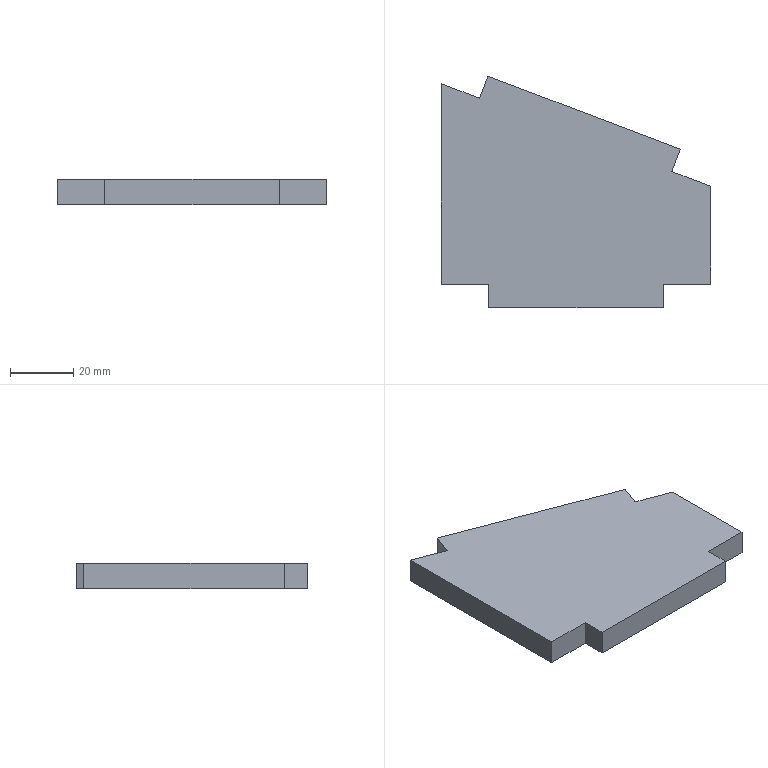Part | SolidWorks | features FlatPattern 1, SMBaseFlange 1, SheetMetal 1 | 1 solid | 14 faces | box 85 x 73.23 x 8 mm | volume 39231 mm3 | plane 14
STEP:
#1=CARTESIAN_POINT('',(162.814,62.221,0.));
#2=VERTEX_POINT('',#1);
#3=CARTESIAN_POINT('',(150.814,66.792,0.));
#4=VERTEX_POINT('',#3);
#5=CARTESIAN_POINT('',(162.814,62.221,0.));
#6=DIRECTION('',(-0.9345,0.3559,0.));
#7=VECTOR('',#6,1000.);
#8=LINE('',#5,#7);
#9=EDGE_CURVE('',#2,#4,#8,.T.);
#10=ORIENTED_EDGE('',*,*,#9,.T.);
#11=CARTESIAN_POINT('',(150.814,66.792,8.));
#12=VERTEX_POINT('',#11);
#13=CARTESIAN_POINT('',(150.814,66.792,8.));
#14=DIRECTION('',(0.,0.,-1.));
#15=VECTOR('',#14,1000.);
#16=LINE('',#13,#15);
#17=EDGE_CURVE('',#12,#4,#16,.T.);
#18=ORIENTED_EDGE('',*,*,#17,.F.);
#19=CARTESIAN_POINT('',(162.814,62.221,8.));
#20=VERTEX_POINT('',#19);
#21=CARTESIAN_POINT('',(162.814,62.221,8.));
#22=DIRECTION('',(-0.9345,0.3559,0.));
#23=VECTOR('',#22,1000.);
#24=LINE('',#21,#23);
#25=EDGE_CURVE('',#20,#12,#24,.T.);
#26=ORIENTED_EDGE('',*,*,#25,.F.);
#27=CARTESIAN_POINT('',(162.814,62.221,8.));
#28=DIRECTION('',(0.,0.,-1.));
#29=VECTOR('',#28,1000.);
#30=LINE('',#27,#29);
#31=EDGE_CURVE('',#20,#2,#30,.T.);
#32=ORIENTED_EDGE('',*,*,#31,.T.);
#33=EDGE_LOOP('',(#10,#18,#26,#32));
#34=FACE_OUTER_BOUND('',#33,.T.);
#35=CARTESIAN_POINT('',(162.814,62.221,8.));
#36=DIRECTION('',(-0.3559,-0.9345,0.));
#37=DIRECTION('',(0.9345,-0.3559,0.));
#38=AXIS2_PLACEMENT_3D('',#35,#36,#37);
#39=PLANE('',#38);
#40=ADVANCED_FACE('',(#34),#39,.F.);
#41=CARTESIAN_POINT('',(150.814,3.5,0.));
#42=VERTEX_POINT('',#41);
#43=CARTESIAN_POINT('',(150.814,66.792,0.));
#44=DIRECTION('',(0.,-1.,0.));
#45=VECTOR('',#44,1000.);
#46=LINE('',#43,#45);
#47=EDGE_CURVE('',#4,#42,#46,.T.);
#48=ORIENTED_EDGE('',*,*,#47,.T.);
#49=CARTESIAN_POINT('',(150.814,3.5,8.));
#50=VERTEX_POINT('',#49);
#51=CARTESIAN_POINT('',(150.814,3.5,8.));
#52=DIRECTION('',(0.,0.,-1.));
#53=VECTOR('',#52,1000.);
#54=LINE('',#51,#53);
#55=EDGE_CURVE('',#50,#42,#54,.T.);
#56=ORIENTED_EDGE('',*,*,#55,.F.);
#57=CARTESIAN_POINT('',(150.814,66.792,8.));
#58=DIRECTION('',(0.,-1.,0.));
#59=VECTOR('',#58,1000.);
#60=LINE('',#57,#59);
#61=EDGE_CURVE('',#12,#50,#60,.T.);
#62=ORIENTED_EDGE('',*,*,#61,.F.);
#63=ORIENTED_EDGE('',*,*,#17,.T.);
#64=EDGE_LOOP('',(#48,#56,#62,#63));
#65=FACE_OUTER_BOUND('',#64,.T.);
#66=CARTESIAN_POINT('',(150.814,66.792,8.));
#67=DIRECTION('',(1.,0.,0.));
#68=DIRECTION('',(0.,0.,-1.));
#69=AXIS2_PLACEMENT_3D('',#66,#67,#68);
#70=PLANE('',#69);
#71=ADVANCED_FACE('',(#65),#70,.F.);
#72=CARTESIAN_POINT('',(165.814,3.5,0.));
#73=VERTEX_POINT('',#72);
#74=CARTESIAN_POINT('',(150.814,3.5,0.));
#75=DIRECTION('',(1.,0.,0.));
#76=VECTOR('',#75,1000.);
#77=LINE('',#74,#76);
#78=EDGE_CURVE('',#42,#73,#77,.T.);
#79=ORIENTED_EDGE('',*,*,#78,.T.);
#80=CARTESIAN_POINT('',(165.814,3.5,8.));
#81=VERTEX_POINT('',#80);
#82=CARTESIAN_POINT('',(165.814,3.5,8.));
#83=DIRECTION('',(0.,0.,-1.));
#84=VECTOR('',#83,1000.);
#85=LINE('',#82,#84);
#86=EDGE_CURVE('',#81,#73,#85,.T.);
#87=ORIENTED_EDGE('',*,*,#86,.F.);
#88=CARTESIAN_POINT('',(150.814,3.5,8.));
#89=DIRECTION('',(1.,0.,0.));
#90=VECTOR('',#89,1000.);
#91=LINE('',#88,#90);
#92=EDGE_CURVE('',#50,#81,#91,.T.);
#93=ORIENTED_EDGE('',*,*,#92,.F.);
#94=ORIENTED_EDGE('',*,*,#55,.T.);
#95=EDGE_LOOP('',(#79,#87,#93,#94));
#96=FACE_OUTER_BOUND('',#95,.T.);
#97=CARTESIAN_POINT('',(150.814,3.5,8.));
#98=DIRECTION('',(0.,1.,0.));
#99=DIRECTION('',(0.,0.,1.));
#100=AXIS2_PLACEMENT_3D('',#97,#98,#99);
#101=PLANE('',#100);
#102=ADVANCED_FACE('',(#96),#101,.F.);
#103=CARTESIAN_POINT('',(165.814,-4.,0.));
#104=VERTEX_POINT('',#103);
#105=CARTESIAN_POINT('',(165.814,-4.,0.));
#106=DIRECTION('',(0.,-1.,0.));
#107=VECTOR('',#106,1000.);
#108=LINE('',#105,#107);
#109=EDGE_CURVE('',#73,#104,#108,.T.);
#110=ORIENTED_EDGE('',*,*,#109,.T.);
#111=CARTESIAN_POINT('',(165.814,-4.,8.));
#112=VERTEX_POINT('',#111);
#113=CARTESIAN_POINT('',(165.814,-4.,8.));
#114=DIRECTION('',(0.,0.,-1.));
#115=VECTOR('',#114,1000.);
#116=LINE('',#113,#115);
#117=EDGE_CURVE('',#112,#104,#116,.T.);
#118=ORIENTED_EDGE('',*,*,#117,.F.);
#119=CARTESIAN_POINT('',(165.814,-4.,8.));
#120=DIRECTION('',(0.,-1.,0.));
#121=VECTOR('',#120,1000.);
#122=LINE('',#119,#121);
#123=EDGE_CURVE('',#81,#112,#122,.T.);
#124=ORIENTED_EDGE('',*,*,#123,.F.);
#125=ORIENTED_EDGE('',*,*,#86,.T.);
#126=EDGE_LOOP('',(#110,#118,#124,#125));
#127=FACE_OUTER_BOUND('',#126,.T.);
#128=CARTESIAN_POINT('',(165.814,-4.,8.));
#129=DIRECTION('',(1.,0.,0.));
#130=DIRECTION('',(0.,0.,-1.));
#131=AXIS2_PLACEMENT_3D('',#128,#129,#130);
#132=PLANE('',#131);
#133=ADVANCED_FACE('',(#127),#132,.F.);
#134=CARTESIAN_POINT('',(220.814,-4.,0.));
#135=VERTEX_POINT('',#134);
#136=CARTESIAN_POINT('',(220.814,-4.,0.));
#137=DIRECTION('',(1.,0.,0.));
#138=VECTOR('',#137,1000.);
#139=LINE('',#136,#138);
#140=EDGE_CURVE('',#104,#135,#139,.T.);
#141=ORIENTED_EDGE('',*,*,#140,.T.);
#142=CARTESIAN_POINT('',(220.814,-4.,8.));
#143=VERTEX_POINT('',#142);
#144=CARTESIAN_POINT('',(220.814,-4.,8.));
#145=DIRECTION('',(0.,0.,-1.));
#146=VECTOR('',#145,1000.);
#147=LINE('',#144,#146);
#148=EDGE_CURVE('',#143,#135,#147,.T.);
#149=ORIENTED_EDGE('',*,*,#148,.F.);
#150=CARTESIAN_POINT('',(220.814,-4.,8.));
#151=DIRECTION('',(1.,0.,0.));
#152=VECTOR('',#151,1000.);
#153=LINE('',#150,#152);
#154=EDGE_CURVE('',#112,#143,#153,.T.);
#155=ORIENTED_EDGE('',*,*,#154,.F.);
#156=ORIENTED_EDGE('',*,*,#117,.T.);
#157=EDGE_LOOP('',(#141,#149,#155,#156));
#158=FACE_OUTER_BOUND('',#157,.T.);
#159=CARTESIAN_POINT('',(220.814,-4.,8.));
#160=DIRECTION('',(0.,1.,0.));
#161=DIRECTION('',(-1.,0.,0.));
#162=AXIS2_PLACEMENT_3D('',#159,#160,#161);
#163=PLANE('',#162);
#164=ADVANCED_FACE('',(#158),#163,.F.);
#165=CARTESIAN_POINT('',(220.814,3.5,0.));
#166=VERTEX_POINT('',#165);
#167=CARTESIAN_POINT('',(220.814,3.5,0.));
#168=DIRECTION('',(0.,1.,0.));
#169=VECTOR('',#168,1000.);
#170=LINE('',#167,#169);
#171=EDGE_CURVE('',#135,#166,#170,.T.);
#172=ORIENTED_EDGE('',*,*,#171,.T.);
#173=CARTESIAN_POINT('',(220.814,3.5,8.));
#174=VERTEX_POINT('',#173);
#175=CARTESIAN_POINT('',(220.814,3.5,8.));
#176=DIRECTION('',(0.,0.,-1.));
#177=VECTOR('',#176,1000.);
#178=LINE('',#175,#177);
#179=EDGE_CURVE('',#174,#166,#178,.T.);
#180=ORIENTED_EDGE('',*,*,#179,.F.);
#181=CARTESIAN_POINT('',(220.814,3.5,8.));
#182=DIRECTION('',(0.,1.,0.));
#183=VECTOR('',#182,1000.);
#184=LINE('',#181,#183);
#185=EDGE_CURVE('',#143,#174,#184,.T.);
#186=ORIENTED_EDGE('',*,*,#185,.F.);
#187=ORIENTED_EDGE('',*,*,#148,.T.);
#188=EDGE_LOOP('',(#172,#180,#186,#187));
#189=FACE_OUTER_BOUND('',#188,.T.);
#190=CARTESIAN_POINT('',(220.814,3.5,8.));
#191=DIRECTION('',(-1.,0.,0.));
#192=DIRECTION('',(0.,0.,1.));
#193=AXIS2_PLACEMENT_3D('',#190,#191,#192);
#194=PLANE('',#193);
#195=ADVANCED_FACE('',(#189),#194,.F.);
#196=CARTESIAN_POINT('',(235.814,3.5,0.));
#197=VERTEX_POINT('',#196);
#198=CARTESIAN_POINT('',(220.814,3.5,0.));
#199=DIRECTION('',(1.,0.,0.));
#200=VECTOR('',#199,1000.);
#201=LINE('',#198,#200);
#202=EDGE_CURVE('',#166,#197,#201,.T.);
#203=ORIENTED_EDGE('',*,*,#202,.T.);
#204=CARTESIAN_POINT('',(235.814,3.5,8.));
#205=VERTEX_POINT('',#204);
#206=CARTESIAN_POINT('',(235.814,3.5,8.));
#207=DIRECTION('',(0.,0.,-1.));
#208=VECTOR('',#207,1000.);
#209=LINE('',#206,#208);
#210=EDGE_CURVE('',#205,#197,#209,.T.);
#211=ORIENTED_EDGE('',*,*,#210,.F.);
#212=CARTESIAN_POINT('',(220.814,3.5,8.));
#213=DIRECTION('',(1.,0.,0.));
#214=VECTOR('',#213,1000.);
#215=LINE('',#212,#214);
#216=EDGE_CURVE('',#174,#205,#215,.T.);
#217=ORIENTED_EDGE('',*,*,#216,.F.);
#218=ORIENTED_EDGE('',*,*,#179,.T.);
#219=EDGE_LOOP('',(#203,#211,#217,#218));
#220=FACE_OUTER_BOUND('',#219,.T.);
#221=CARTESIAN_POINT('',(220.814,3.5,8.));
#222=DIRECTION('',(0.,1.,0.));
#223=DIRECTION('',(0.,0.,1.));
#224=AXIS2_PLACEMENT_3D('',#221,#222,#223);
#225=PLANE('',#224);
#226=ADVANCED_FACE('',(#220),#225,.F.);
#227=CARTESIAN_POINT('',(235.814,34.418,0.));
#228=VERTEX_POINT('',#227);
#229=CARTESIAN_POINT('',(235.814,3.5,0.));
#230=DIRECTION('',(0.,1.,0.));
#231=VECTOR('',#230,1000.);
#232=LINE('',#229,#231);
#233=EDGE_CURVE('',#197,#228,#232,.T.);
#234=ORIENTED_EDGE('',*,*,#233,.T.);
#235=CARTESIAN_POINT('',(235.814,34.418,8.));
#236=VERTEX_POINT('',#235);
#237=CARTESIAN_POINT('',(235.814,34.418,8.));
#238=DIRECTION('',(0.,0.,-1.));
#239=VECTOR('',#238,1000.);
#240=LINE('',#237,#239);
#241=EDGE_CURVE('',#236,#228,#240,.T.);
#242=ORIENTED_EDGE('',*,*,#241,.F.);
#243=CARTESIAN_POINT('',(235.814,3.5,8.));
#244=DIRECTION('',(0.,1.,0.));
#245=VECTOR('',#244,1000.);
#246=LINE('',#243,#245);
#247=EDGE_CURVE('',#205,#236,#246,.T.);
#248=ORIENTED_EDGE('',*,*,#247,.F.);
#249=ORIENTED_EDGE('',*,*,#210,.T.);
#250=EDGE_LOOP('',(#234,#242,#248,#249));
#251=FACE_OUTER_BOUND('',#250,.T.);
#252=CARTESIAN_POINT('',(235.814,3.5,8.));
#253=DIRECTION('',(-1.,0.,0.));
#254=DIRECTION('',(0.,0.,1.));
#255=AXIS2_PLACEMENT_3D('',#252,#253,#254);
#256=PLANE('',#255);
#257=ADVANCED_FACE('',(#251),#256,.F.);
#258=CARTESIAN_POINT('',(223.557,39.086,0.));
#259=VERTEX_POINT('',#258);
#260=CARTESIAN_POINT('',(235.814,34.418,0.));
#261=DIRECTION('',(-0.9345,0.3559,0.));
#262=VECTOR('',#261,1000.);
#263=LINE('',#260,#262);
#264=EDGE_CURVE('',#228,#259,#263,.T.);
#265=ORIENTED_EDGE('',*,*,#264,.T.);
#266=CARTESIAN_POINT('',(223.557,39.086,8.));
#267=VERTEX_POINT('',#266);
#268=CARTESIAN_POINT('',(223.557,39.086,8.));
#269=DIRECTION('',(0.,0.,-1.));
#270=VECTOR('',#269,1000.);
#271=LINE('',#268,#270);
#272=EDGE_CURVE('',#267,#259,#271,.T.);
#273=ORIENTED_EDGE('',*,*,#272,.F.);
#274=CARTESIAN_POINT('',(235.814,34.418,8.));
#275=DIRECTION('',(-0.9345,0.3559,0.));
#276=VECTOR('',#275,1000.);
#277=LINE('',#274,#276);
#278=EDGE_CURVE('',#236,#267,#277,.T.);
#279=ORIENTED_EDGE('',*,*,#278,.F.);
#280=ORIENTED_EDGE('',*,*,#241,.T.);
#281=EDGE_LOOP('',(#265,#273,#279,#280));
#282=FACE_OUTER_BOUND('',#281,.T.);
#283=CARTESIAN_POINT('',(235.814,34.418,8.));
#284=DIRECTION('',(-0.3559,-0.9345,0.));
#285=DIRECTION('',(0.9345,-0.3559,0.));
#286=AXIS2_PLACEMENT_3D('',#283,#284,#285);
#287=PLANE('',#286);
#288=ADVANCED_FACE('',(#282),#287,.F.);
#289=CARTESIAN_POINT('',(226.227,46.095,0.));
#290=VERTEX_POINT('',#289);
#291=CARTESIAN_POINT('',(223.557,39.086,0.));
#292=DIRECTION('',(0.3559,0.9345,0.));
#293=VECTOR('',#292,1000.);
#294=LINE('',#291,#293);
#295=EDGE_CURVE('',#259,#290,#294,.T.);
#296=ORIENTED_EDGE('',*,*,#295,.T.);
#297=CARTESIAN_POINT('',(226.227,46.095,8.));
#298=VERTEX_POINT('',#297);
#299=CARTESIAN_POINT('',(226.227,46.095,8.));
#300=DIRECTION('',(0.,0.,-1.));
#301=VECTOR('',#300,1000.);
#302=LINE('',#299,#301);
#303=EDGE_CURVE('',#298,#290,#302,.T.);
#304=ORIENTED_EDGE('',*,*,#303,.F.);
#305=CARTESIAN_POINT('',(223.557,39.086,8.));
#306=DIRECTION('',(0.3559,0.9345,0.));
#307=VECTOR('',#306,1000.);
#308=LINE('',#305,#307);
#309=EDGE_CURVE('',#267,#298,#308,.T.);
#310=ORIENTED_EDGE('',*,*,#309,.F.);
#311=ORIENTED_EDGE('',*,*,#272,.T.);
#312=EDGE_LOOP('',(#296,#304,#310,#311));
#313=FACE_OUTER_BOUND('',#312,.T.);
#314=CARTESIAN_POINT('',(223.557,39.086,8.));
#315=DIRECTION('',(-0.9345,0.3559,0.));
#316=DIRECTION('',(-0.3559,-0.9345,0.));
#317=AXIS2_PLACEMENT_3D('',#314,#315,#316);
#318=PLANE('',#317);
#319=ADVANCED_FACE('',(#313),#318,.F.);
#320=CARTESIAN_POINT('',(165.483,69.23,0.));
#321=VERTEX_POINT('',#320);
#322=CARTESIAN_POINT('',(226.227,46.095,0.));
#323=DIRECTION('',(-0.9345,0.3559,0.));
#324=VECTOR('',#323,1000.);
#325=LINE('',#322,#324);
#326=EDGE_CURVE('',#290,#321,#325,.T.);
#327=ORIENTED_EDGE('',*,*,#326,.T.);
#328=CARTESIAN_POINT('',(165.483,69.23,8.));
#329=VERTEX_POINT('',#328);
#330=CARTESIAN_POINT('',(165.483,69.23,8.));
#331=DIRECTION('',(0.,0.,-1.));
#332=VECTOR('',#331,1000.);
#333=LINE('',#330,#332);
#334=EDGE_CURVE('',#329,#321,#333,.T.);
#335=ORIENTED_EDGE('',*,*,#334,.F.);
#336=CARTESIAN_POINT('',(226.227,46.095,8.));
#337=DIRECTION('',(-0.9345,0.3559,0.));
#338=VECTOR('',#337,1000.);
#339=LINE('',#336,#338);
#340=EDGE_CURVE('',#298,#329,#339,.T.);
#341=ORIENTED_EDGE('',*,*,#340,.F.);
#342=ORIENTED_EDGE('',*,*,#303,.T.);
#343=EDGE_LOOP('',(#327,#335,#341,#342));
#344=FACE_OUTER_BOUND('',#343,.T.);
#345=CARTESIAN_POINT('',(226.227,46.095,8.));
#346=DIRECTION('',(-0.3559,-0.9345,0.));
#347=DIRECTION('',(0.9345,-0.3559,0.));
#348=AXIS2_PLACEMENT_3D('',#345,#346,#347);
#349=PLANE('',#348);
#350=ADVANCED_FACE('',(#344),#349,.F.);
#351=CARTESIAN_POINT('',(165.483,69.23,0.));
#352=DIRECTION('',(-0.3559,-0.9345,0.));
#353=VECTOR('',#352,1000.);
#354=LINE('',#351,#353);
#355=EDGE_CURVE('',#321,#2,#354,.T.);
#356=ORIENTED_EDGE('',*,*,#355,.T.);
#357=ORIENTED_EDGE('',*,*,#31,.F.);
#358=CARTESIAN_POINT('',(165.483,69.23,8.));
#359=DIRECTION('',(-0.3559,-0.9345,0.));
#360=VECTOR('',#359,1000.);
#361=LINE('',#358,#360);
#362=EDGE_CURVE('',#329,#20,#361,.T.);
#363=ORIENTED_EDGE('',*,*,#362,.F.);
#364=ORIENTED_EDGE('',*,*,#334,.T.);
#365=EDGE_LOOP('',(#356,#357,#363,#364));
#366=FACE_OUTER_BOUND('',#365,.T.);
#367=CARTESIAN_POINT('',(165.483,69.23,8.));
#368=DIRECTION('',(0.9345,-0.3559,0.));
#369=DIRECTION('',(0.3559,0.9345,0.));
#370=AXIS2_PLACEMENT_3D('',#367,#368,#369);
#371=PLANE('',#370);
#372=ADVANCED_FACE('',(#366),#371,.F.);
#373=ORIENTED_EDGE('',*,*,#25,.T.);
#374=ORIENTED_EDGE('',*,*,#61,.T.);
#375=ORIENTED_EDGE('',*,*,#92,.T.);
#376=ORIENTED_EDGE('',*,*,#123,.T.);
#377=ORIENTED_EDGE('',*,*,#154,.T.);
#378=ORIENTED_EDGE('',*,*,#185,.T.);
#379=ORIENTED_EDGE('',*,*,#216,.T.);
#380=ORIENTED_EDGE('',*,*,#247,.T.);
#381=ORIENTED_EDGE('',*,*,#278,.T.);
#382=ORIENTED_EDGE('',*,*,#309,.T.);
#383=ORIENTED_EDGE('',*,*,#340,.T.);
#384=ORIENTED_EDGE('',*,*,#362,.T.);
#385=EDGE_LOOP('',(#373,#374,#375,#376,#377,#378,#379,#380,#381,#382,#383,#384));
#386=FACE_OUTER_BOUND('',#385,.T.);
#387=CARTESIAN_POINT('',(0.,0.,8.));
#388=DIRECTION('',(0.,0.,-1.));
#389=DIRECTION('',(-1.,0.,0.));
#390=AXIS2_PLACEMENT_3D('',#387,#388,#389);
#391=PLANE('',#390);
#392=ADVANCED_FACE('',(#386),#391,.F.);
#393=ORIENTED_EDGE('',*,*,#9,.F.);
#394=ORIENTED_EDGE('',*,*,#355,.F.);
#395=ORIENTED_EDGE('',*,*,#326,.F.);
#396=ORIENTED_EDGE('',*,*,#295,.F.);
#397=ORIENTED_EDGE('',*,*,#264,.F.);
#398=ORIENTED_EDGE('',*,*,#233,.F.);
#399=ORIENTED_EDGE('',*,*,#202,.F.);
#400=ORIENTED_EDGE('',*,*,#171,.F.);
#401=ORIENTED_EDGE('',*,*,#140,.F.);
#402=ORIENTED_EDGE('',*,*,#109,.F.);
#403=ORIENTED_EDGE('',*,*,#78,.F.);
#404=ORIENTED_EDGE('',*,*,#47,.F.);
#405=EDGE_LOOP('',(#393,#394,#395,#396,#397,#398,#399,#400,#401,#402,#403,#404));
#406=FACE_OUTER_BOUND('',#405,.T.);
#407=CARTESIAN_POINT('',(0.,0.,0.));
#408=DIRECTION('',(0.,0.,-1.));
#409=DIRECTION('',(-1.,0.,0.));
#410=AXIS2_PLACEMENT_3D('',#407,#408,#409);
#411=PLANE('',#410);
#412=ADVANCED_FACE('',(#406),#411,.T.);
#413=CLOSED_SHELL('',(#40,#71,#102,#133,#164,#195,#226,#257,#288,#319,#350,#372,#392,#412));
#414=MANIFOLD_SOLID_BREP('',#413);
#415=CARTESIAN_POINT('',(0.,0.,0.));
#416=DIRECTION('',(0.,0.,1.));
#417=DIRECTION('',(1.,0.,0.));
#418=AXIS2_PLACEMENT_3D('',#415,#416,#417);
#419=(LENGTH_UNIT()NAMED_UNIT(*)SI_UNIT(.MILLI.,.METRE.));
#420=UNCERTAINTY_MEASURE_WITH_UNIT(LENGTH_MEASURE(0.00001),#419,'','');
#421=(NAMED_UNIT(*)PLANE_ANGLE_UNIT()SI_UNIT($,.RADIAN.));
#422=(NAMED_UNIT(*)SI_UNIT($,.STERADIAN.)SOLID_ANGLE_UNIT());
#423=(GEOMETRIC_REPRESENTATION_CONTEXT(3)GLOBAL_UNCERTAINTY_ASSIGNED_CONTEXT((#420))GLOBAL_UNIT_ASSIGNED_CONTEXT((#419,#421,#422))REPRESENTATION_CONTEXT('',''));
#424=ADVANCED_BREP_SHAPE_REPRESENTATION('',(#414,#418),#423);